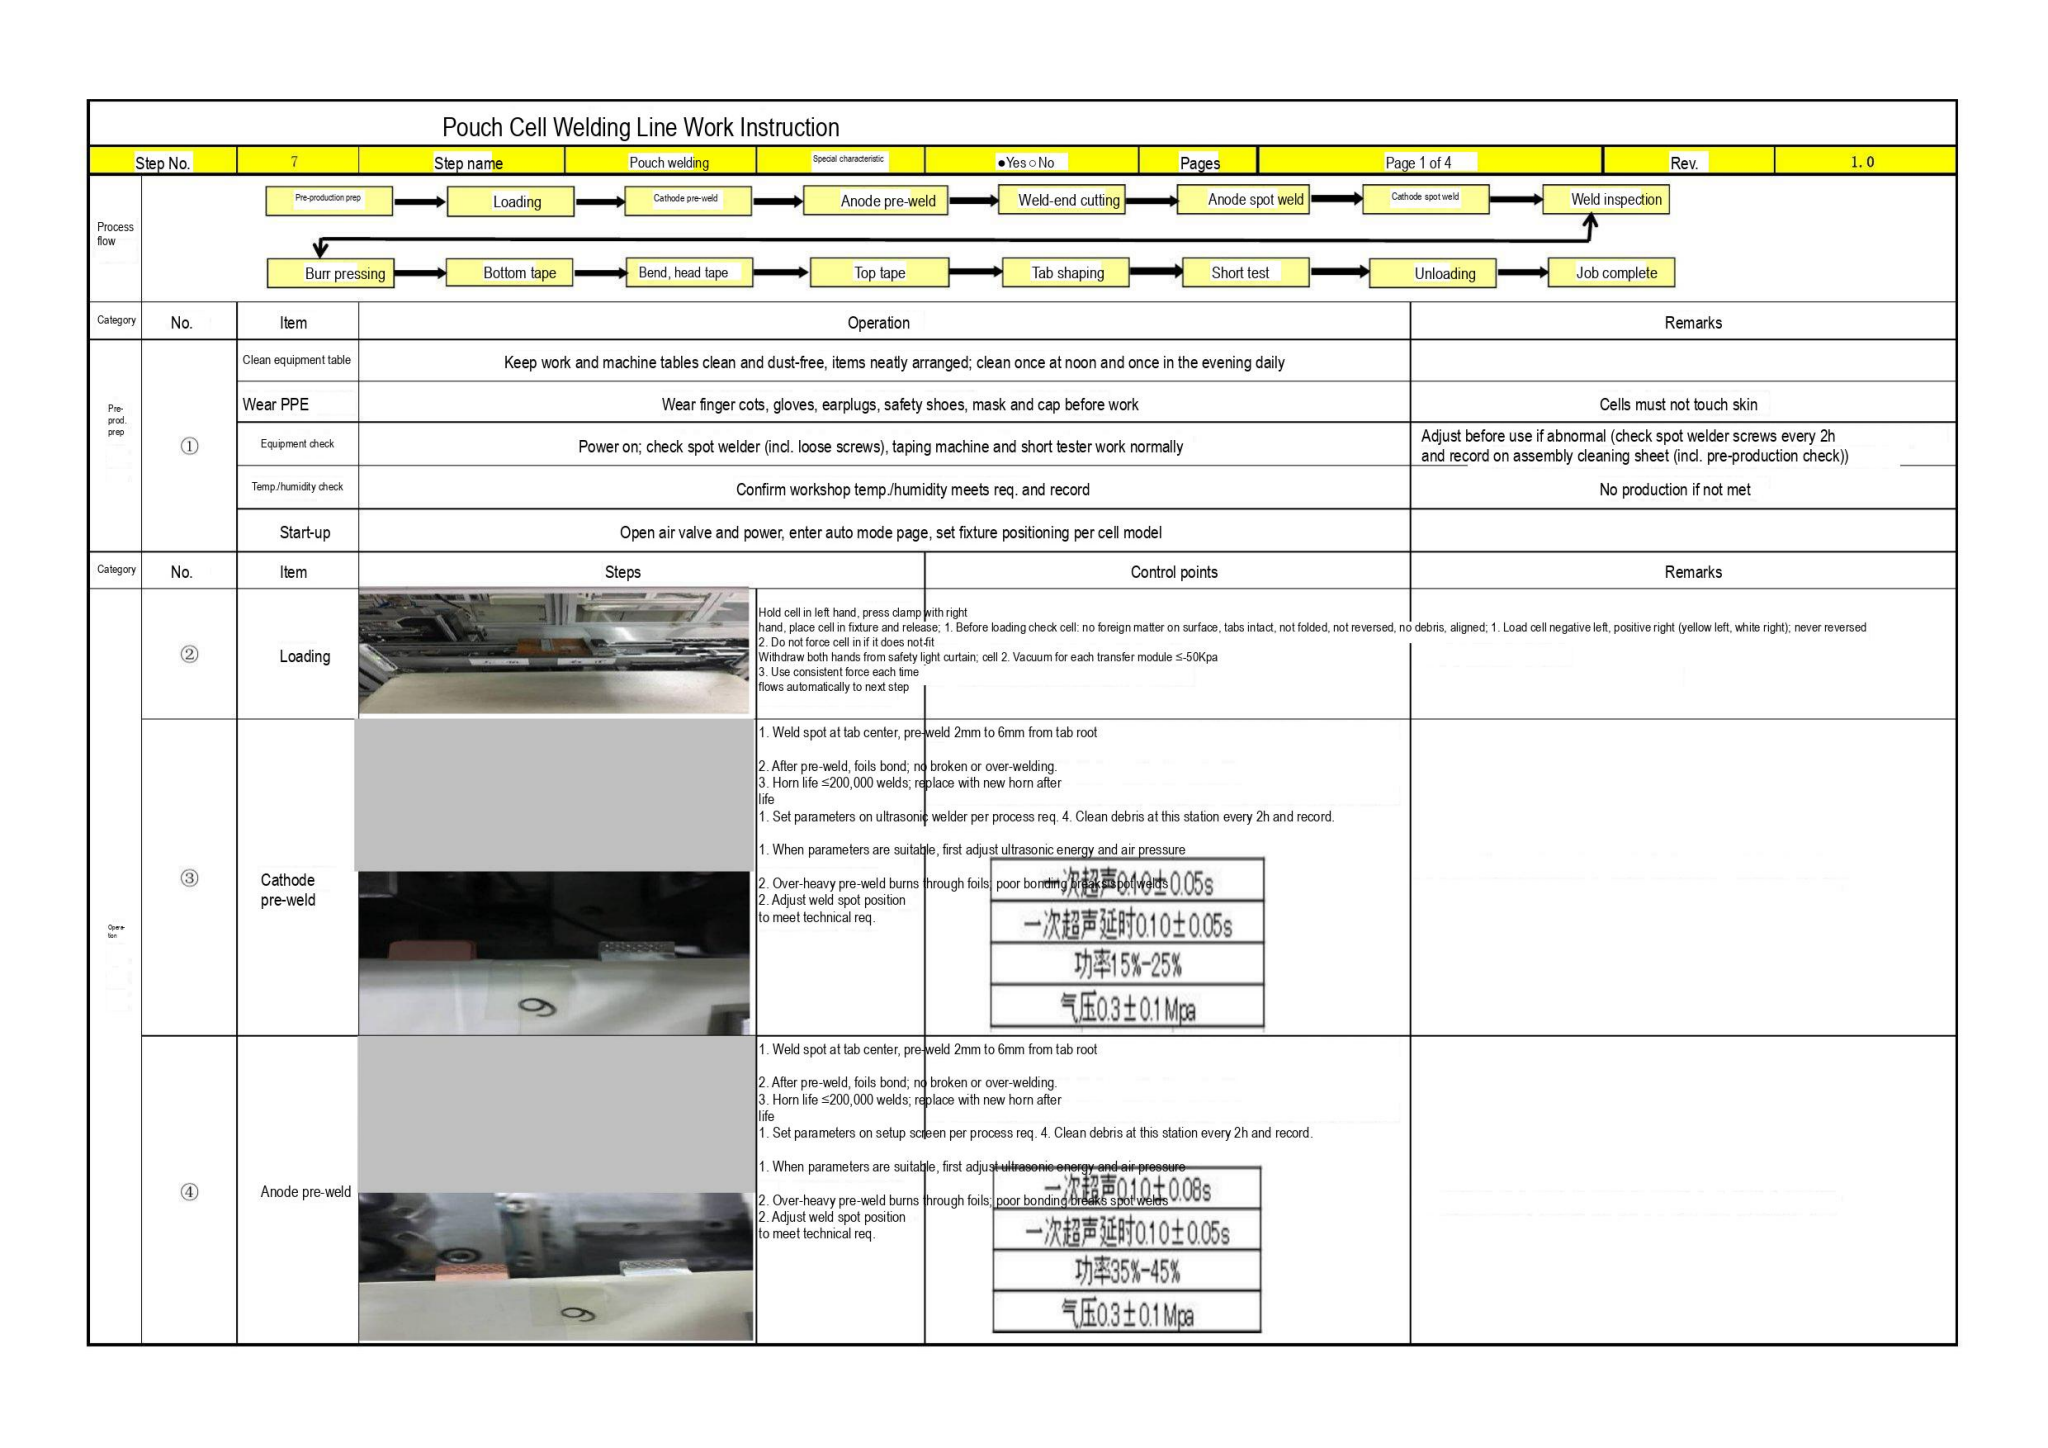# Pouch Cell Welding Line Work Instruction

| Step No. | 7 | Step name | Pouch welding | Special characteristic | ●Yes○No | Pages | Page 1 of 4 | Rev. | 1.0 |
|---|---|---|---|---|---|---|---|---|---|

Process flow

Pre-production prep → Loading → Cathode pre-weld → Anode pre-weld → Weld-end cutting → Anode spot weld → Cathode spot weld → Weld inspection

Burr pressing → Bottom tape → Bend, head tape → Top tape → Tab shaping → Short test → Unloading → Job complete

| Category | No. | Item | Operation | Remarks |
|---|---|---|---|---|
| Pre-prod. prep | ① | Clean equipment table | Keep work and machine tables clean and dust-free, items neatly arranged; clean once at noon and once in the evening daily | |
| | | Wear PPE | Wear finger cots, gloves, earplugs, safety shoes, mask and cap before work | Cells must not touch skin |
| | | Equipment check | Power on; check spot welder (incl. loose screws), taping machine and short tester work normally | Adjust before use if abnormal (check spot welder screws every 2h and record on assembly cleaning sheet (incl. pre-production check)) |
| | | Temp./humidity check | Confirm workshop temp./humidity meets req. and record | No production if not met |
| | | Start-up | Open air valve and power, enter auto mode page, set fixture positioning per cell model | |

| Category | No. | Item | Steps | Control points | Remarks |
|---|---|---|---|---|---|
| Opera-tion | ② | Loading | Hold cell in left hand, press clamp with right<br>hand, place cell in fixture and release; 1. Before loading check cell: no foreign matter on surface, tabs intact, not folded, not reversed, no debris, aligned; 1. Load cell negative left, positive right (yellow left, white right); never reversed<br>2. Do not force cell in if it does not fit<br>Withdraw both hands from safety light curtain; cell 2. Vacuum for each transfer module ≤-50Kpa<br>3. Use consistent force each time<br>flows automatically to next step | | |
| | ③ | Cathode pre-weld | 1. Weld spot at tab center, pre-weld 2mm to 6mm from tab root<br>2. After pre-weld, foils bond; no broken or over-welding.<br>3. Horn life ≤200,000 welds; replace with new horn after life<br>1. Set parameters on ultrasonic welder per process req. 4. Clean debris at this station every 2h and record.<br>1. When parameters are suitable, first adjust ultrasonic energy and air pressure<br>2. Over-heavy pre-weld burns through foils; poor bonding breaks spot welds<br>2. Adjust weld spot position to meet technical req. | 一次超声0.10±0.05s<br>一次超声延时0.10±0.05s<br>功率15%-25%<br>气压0.3±0.1Mpa | |
| | ④ | Anode pre-weld | 1. Weld spot at tab center, pre-weld 2mm to 6mm from tab root<br>2. After pre-weld, foils bond; no broken or over-welding.<br>3. Horn life ≤200,000 welds; replace with new horn after life<br>1. Set parameters on setup screen per process req. 4. Clean debris at this station every 2h and record.<br>1. When parameters are suitable, first adjust ultrasonic energy and air pressure<br>2. Over-heavy pre-weld burns through foils; poor bonding breaks spot welds<br>2. Adjust weld spot position to meet technical req. | 一次超声0.10±0.08s<br>一次超声延时0.10±0.05s<br>功率35%-45%<br>气压0.3±0.1Mpa | |
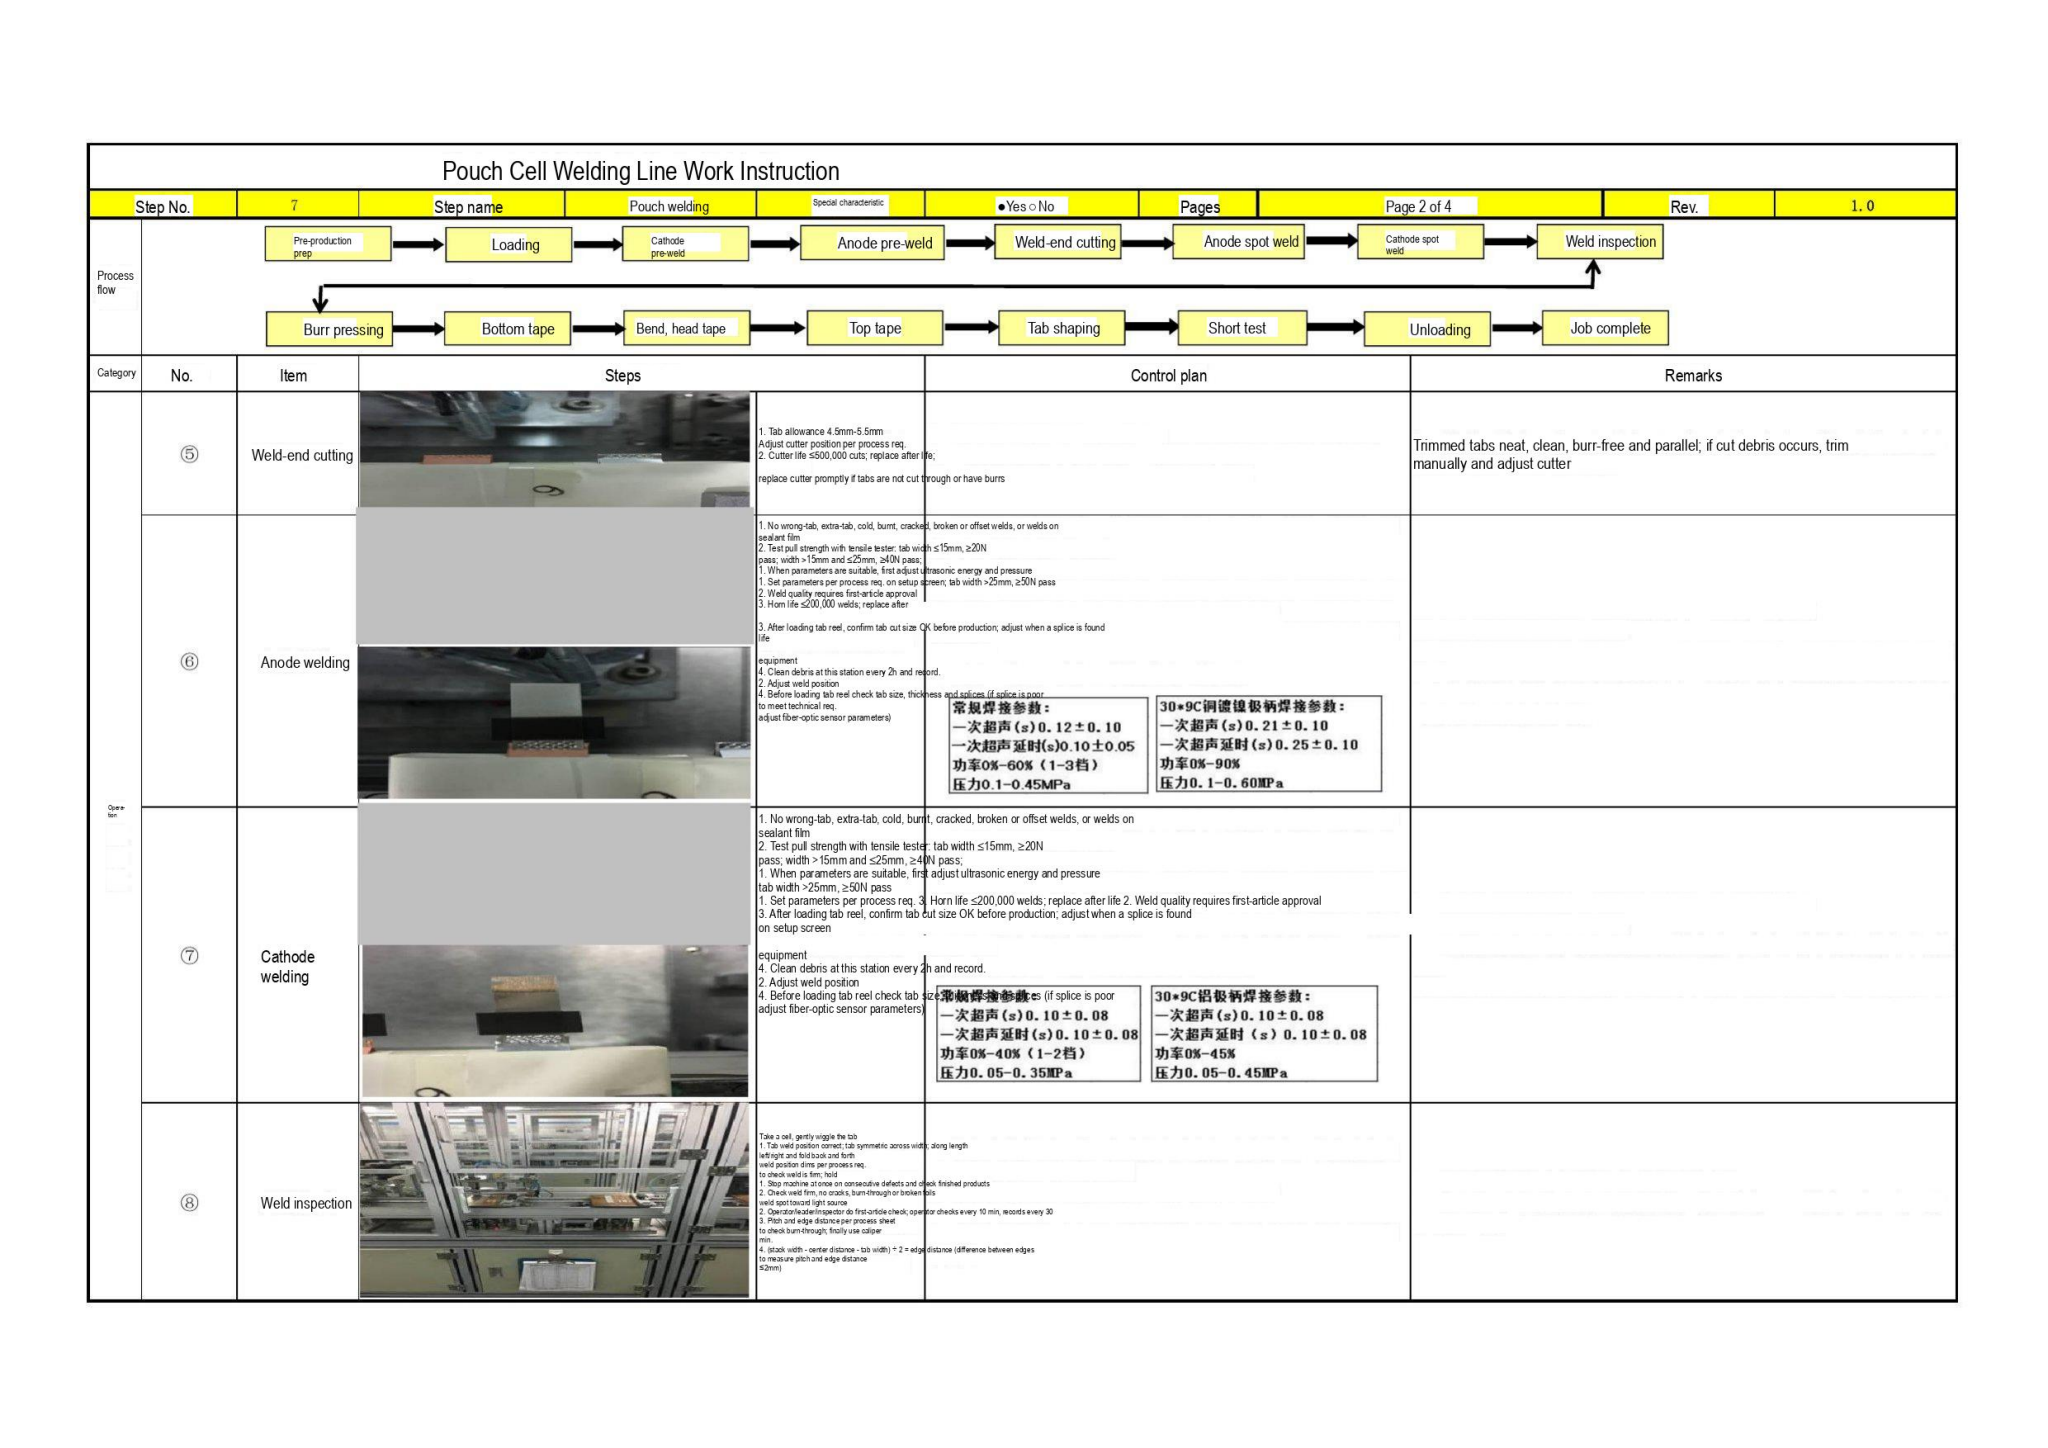Pouch Cell Welding Line Work Instruction

| Step No. | 7 | Step name | Pouch welding | Special characteristic | ●Yes ○No | Pages | Page 2 of 4 | Rev. | 1.0 |
|---|---|---|---|---|---|---|---|---|---|

Process flow

Pre-production prep → Loading → Cathode pre-weld → Anode pre-weld → Weld-end cutting → Anode spot weld → Cathode spot weld → Weld inspection → Burr pressing → Bottom tape → Bend, head tape → Top tape → Tab shaping → Short test → Unloading → Job complete

| Category | No. | Item | Steps | Control plan | Remarks |
|---|---|---|---|---|---|
| Operation | ⑤ | Weld-end cutting | | 1. Tab allowance 4.5mm-5.5mm<br>Adjust cutter position per process req.<br>2. Cutter life ≤500,000 cuts; replace after life;<br><br>replace cutter promptly if tabs are not cut through or have burrs | Trimmed tabs neat, clean, burr-free and parallel; if cut debris occurs, trim manually and adjust cutter |
| | ⑥ | Anode welding | | 1. No wrong-tab, extra-tab, cold, burnt, cracked, broken or offset welds, or welds on sealant film<br>2. Test pull strength with tensile tester: tab width ≤15mm, ≥20N pass; width >15mm and ≤25mm, ≥40N pass;<br>1. When parameters are suitable, first adjust ultrasonic energy and pressure<br>1. Set parameters per process req. on setup screen; tab width >25mm, ≥50N pass<br>2. Weld quality requires first-article approval<br>3. Horn life ≤200,000 welds; replace after<br><br>3. After loading tab reel, confirm tab cut size OK before production; adjust when a splice is found<br>life<br><br>equipment<br>4. Clean debris at this station every 2h and record.<br>2. Adjust weld position<br>4. Before loading tab reel check tab size, thickness and splices (if splice is poor<br>to meet technical req.<br>adjust fiber-optic sensor parameters)<br><br>常规焊接参数：<br>一次超声(s)0.12±0.10<br>一次超声延时(s)0.10±0.05<br>功率0%-60%（1-3档）<br>压力0.1-0.45MPa<br><br>30*9C铜镀镍极柄焊接参数：<br>一次超声(s)0.21±0.10<br>一次超声延时(s)0.25±0.10<br>功率0%-90%<br>压力0.1-0.60MPa | |
| | ⑦ | Cathode welding | | 1. No wrong-tab, extra-tab, cold, burnt, cracked, broken or offset welds, or welds on sealant film<br>2. Test pull strength with tensile tester: tab width ≤15mm, ≥20N pass; width >15mm and ≤25mm, ≥40N pass;<br>1. When parameters are suitable, first adjust ultrasonic energy and pressure<br>tab width >25mm, ≥50N pass<br>1. Set parameters per process req. 3. Horn life ≤200,000 welds; replace after life 2. Weld quality requires first-article approval<br>3. After loading tab reel, confirm tab cut size OK before production; adjust when a splice is found<br>on setup screen<br><br>equipment<br>4. Clean debris at this station every 2h and record.<br>2. Adjust weld position<br>4. Before loading tab reel check tab size (if splice is poor<br>adjust fiber-optic sensor parameters)<br><br>常规焊接参数：<br>一次超声(s)0.10±0.08<br>一次超声延时(s)0.10±0.08<br>功率0%-40%（1-2档）<br>压力0.05-0.35MPa<br><br>30*9C铝极柄焊接参数：<br>一次超声(s)0.10±0.08<br>一次超声延时（s）0.10±0.08<br>功率0%-45%<br>压力0.05-0.45MPa | |
| | ⑧ | Weld inspection | | Take a cell, gently wiggle the tab<br>1. Tab weld position correct; tab symmetric across width; along length<br>left/right and fold back and forth<br>weld position dims per process req.<br>to check weld is firm; hold<br>1. Stop machine at once on consecutive defects and check finished products<br>2. Check weld firm, no cracks, burn-through or broken foils<br>weld spot toward light source<br>2. Operator/leader/inspector do first-article check; operator checks every 10 min, records every 30<br>3. Pitch and edge distance per process sheet<br>to check burn-through; finally use caliper<br>min.<br>4. (stack width - center distance - tab width) ÷ 2 = edge distance (difference between edges<br>to measure pitch and edge distance<br>≤2mm) | |
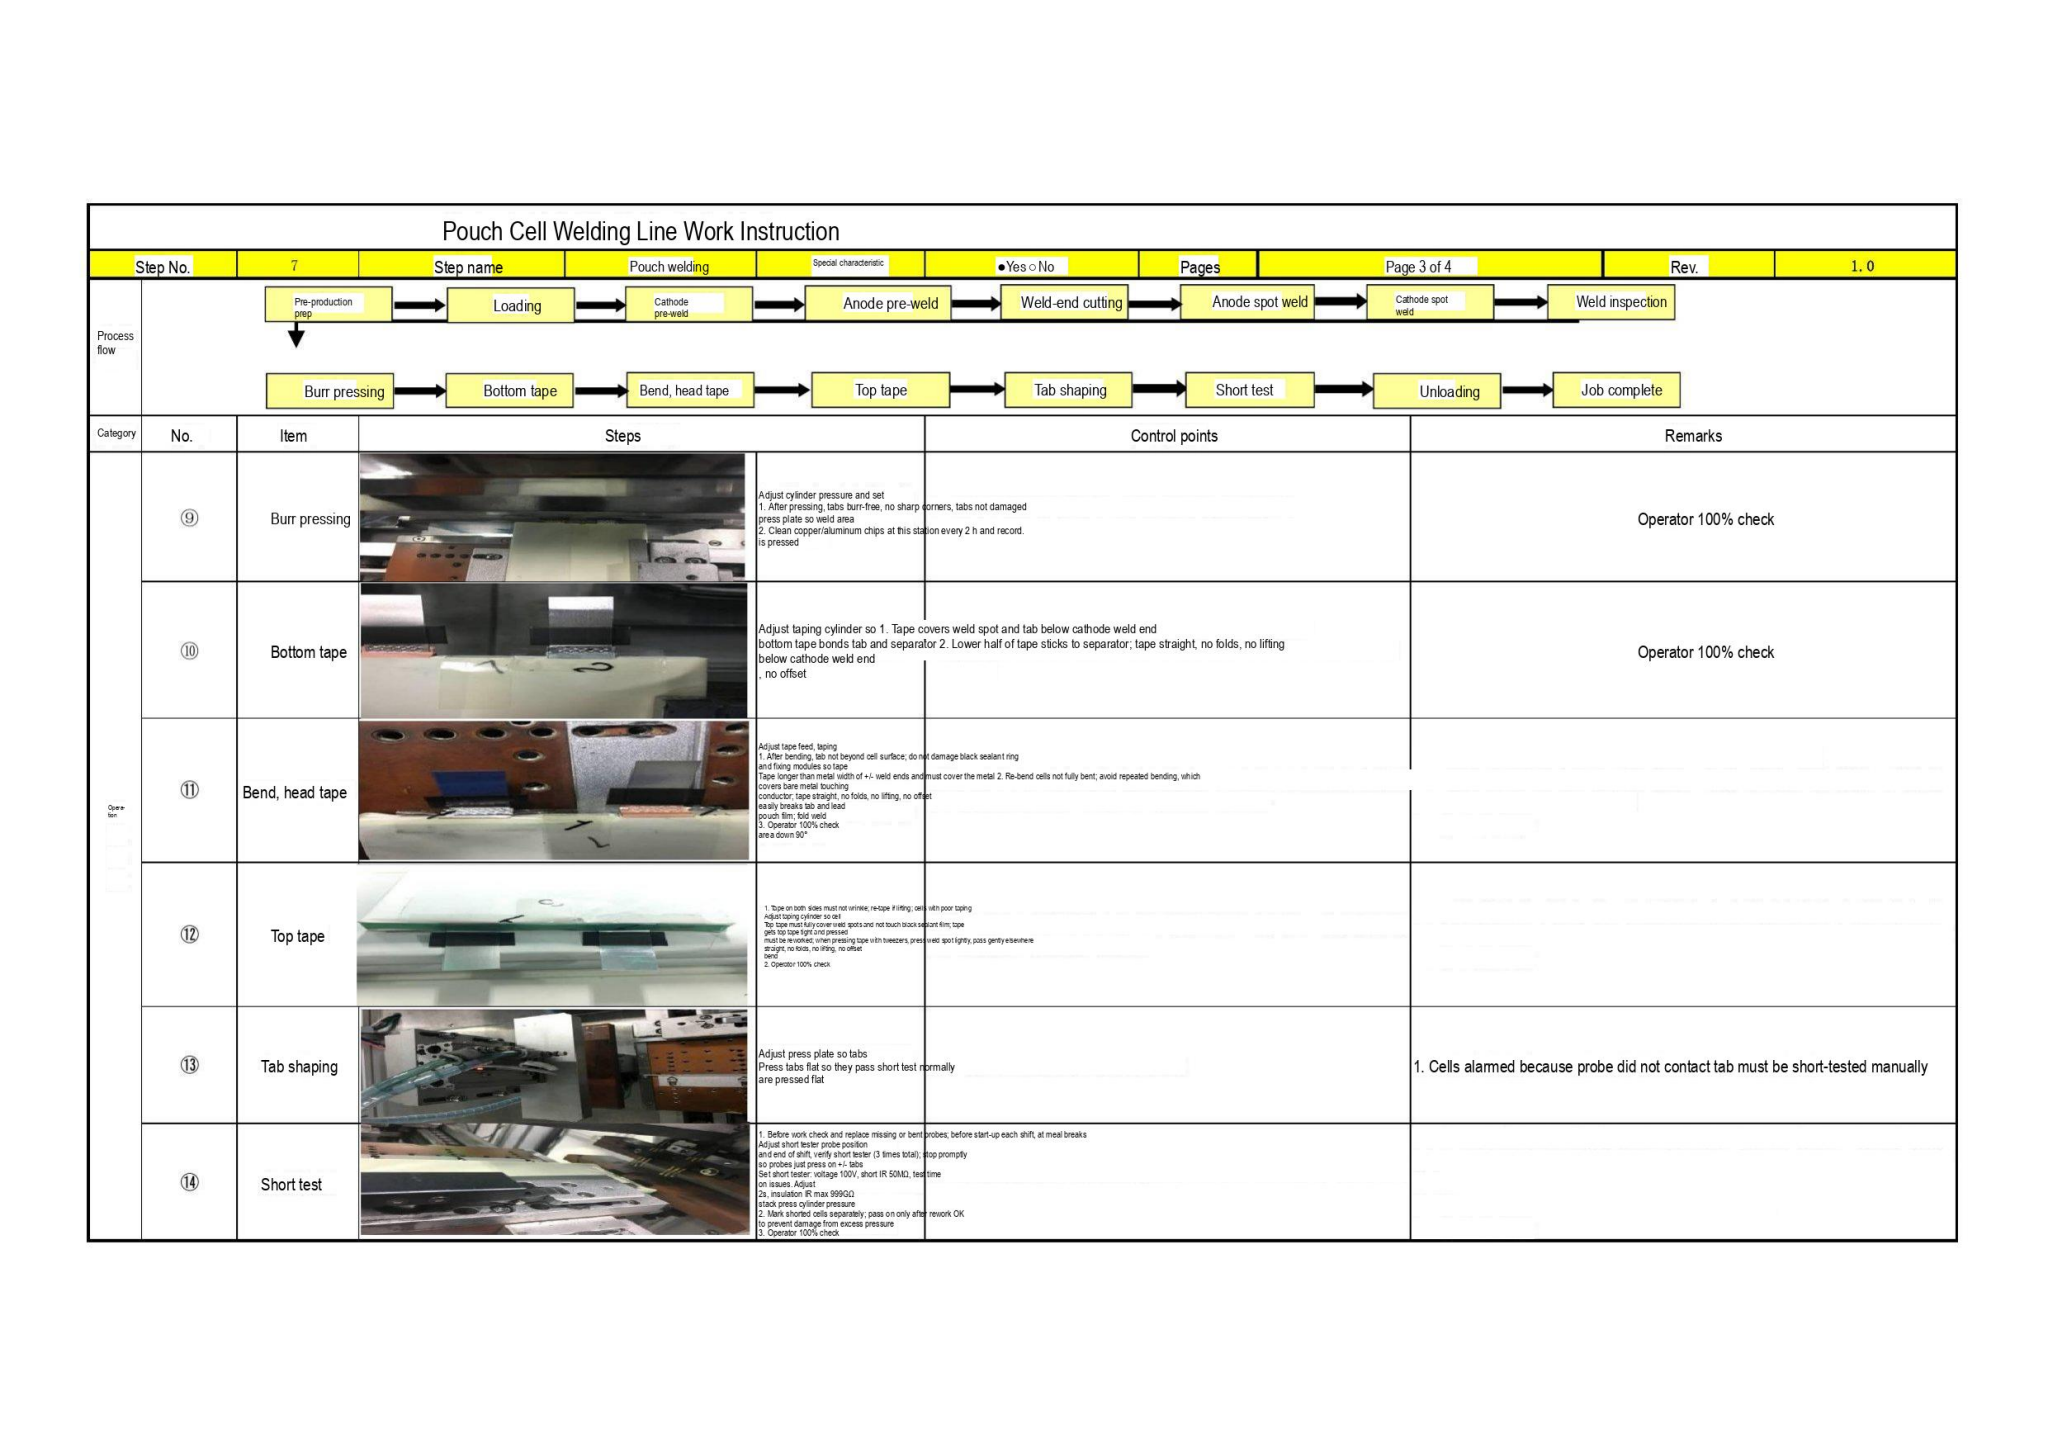Pouch Cell Welding Line Work Instruction

| Step No. | 7 | Step name | Pouch welding | Special characteristic | ●Yes ○No | Pages | Page 3 of 4 | Rev. | 1. 0 |
|---|---|---|---|---|---|---|---|---|---|

Process flow

Pre-production prep → Loading → Cathode pre-weld → Anode pre-weld → Weld-end cutting → Anode spot weld → Cathode spot weld → Weld inspection

Burr pressing → Bottom tape → Bend, head tape → Top tape → Tab shaping → Short test → Unloading → Job complete

| Category | No. | Item | Steps | Control points | Remarks |
|---|---|---|---|---|---|
| Operation | ⑨ | Burr pressing | Adjust cylinder pressure and set press plate so weld area is pressed | 1. After pressing, tabs burr-free, no sharp corners, tabs not damaged<br>2. Clean copper/aluminum chips at this station every 2 h and record. | Operator 100% check |
| | ⑩ | Bottom tape | Adjust taping cylinder so bottom tape bonds tab and separator below cathode weld end, no offset | 1. Tape covers weld spot and tab below cathode weld end<br>2. Lower half of tape sticks to separator; tape straight, no folds, no lifting | Operator 100% check |
| | ⑪ | Bend, head tape | Adjust tape feed, taping and fixing modules so tape covers bare metal touching conductor; tape straight, no folds, no lifting, no offset<br>Tape longer than metal width of +/- weld ends and pouch film; fold weld area down 90° | 1. After bending, tab not beyond cell surface; do not damage black sealant ring<br>must cover the metal 2. Re-bend cells not fully bent; avoid repeated bending, which easily breaks tab and lead<br>3. Operator 100% check | |
| | ⑫ | Top tape | Adjust taping cylinder so cell gets top tape tight and pressed straight, no folds, no lifting, no offset | 1. Tape on both sides must not wrinkle; re-tape if lifting; cells with poor taping must be reworked; when pressing tape with tweezers, press weld spot lightly, pass gently elsewhere<br>Top tape must fully cover weld spots and not touch black sealant film; tape bend<br>2. Operator 100% check | |
| | ⑬ | Tab shaping | Adjust press plate so tabs are pressed flat | Press tabs flat so they pass short test normally | 1. Cells alarmed because probe did not contact tab must be short-tested manually |
| | ⑭ | Short test | Adjust short tester probe position so probes just press on +/- tabs<br>Set short tester: voltage 100V, short IR 50MΩ, test time 2s, insulation IR max 999GΩ<br>Adjust stack press cylinder pressure to prevent damage from excess pressure | 1. Before work check and replace missing or bent probes; before start-up each shift, at meal breaks and end of shift, verify short tester (3 times total); stop promptly on issues.<br>2. Mark shorted cells separately; pass on only after rework OK<br>3. Operator 100% check | |
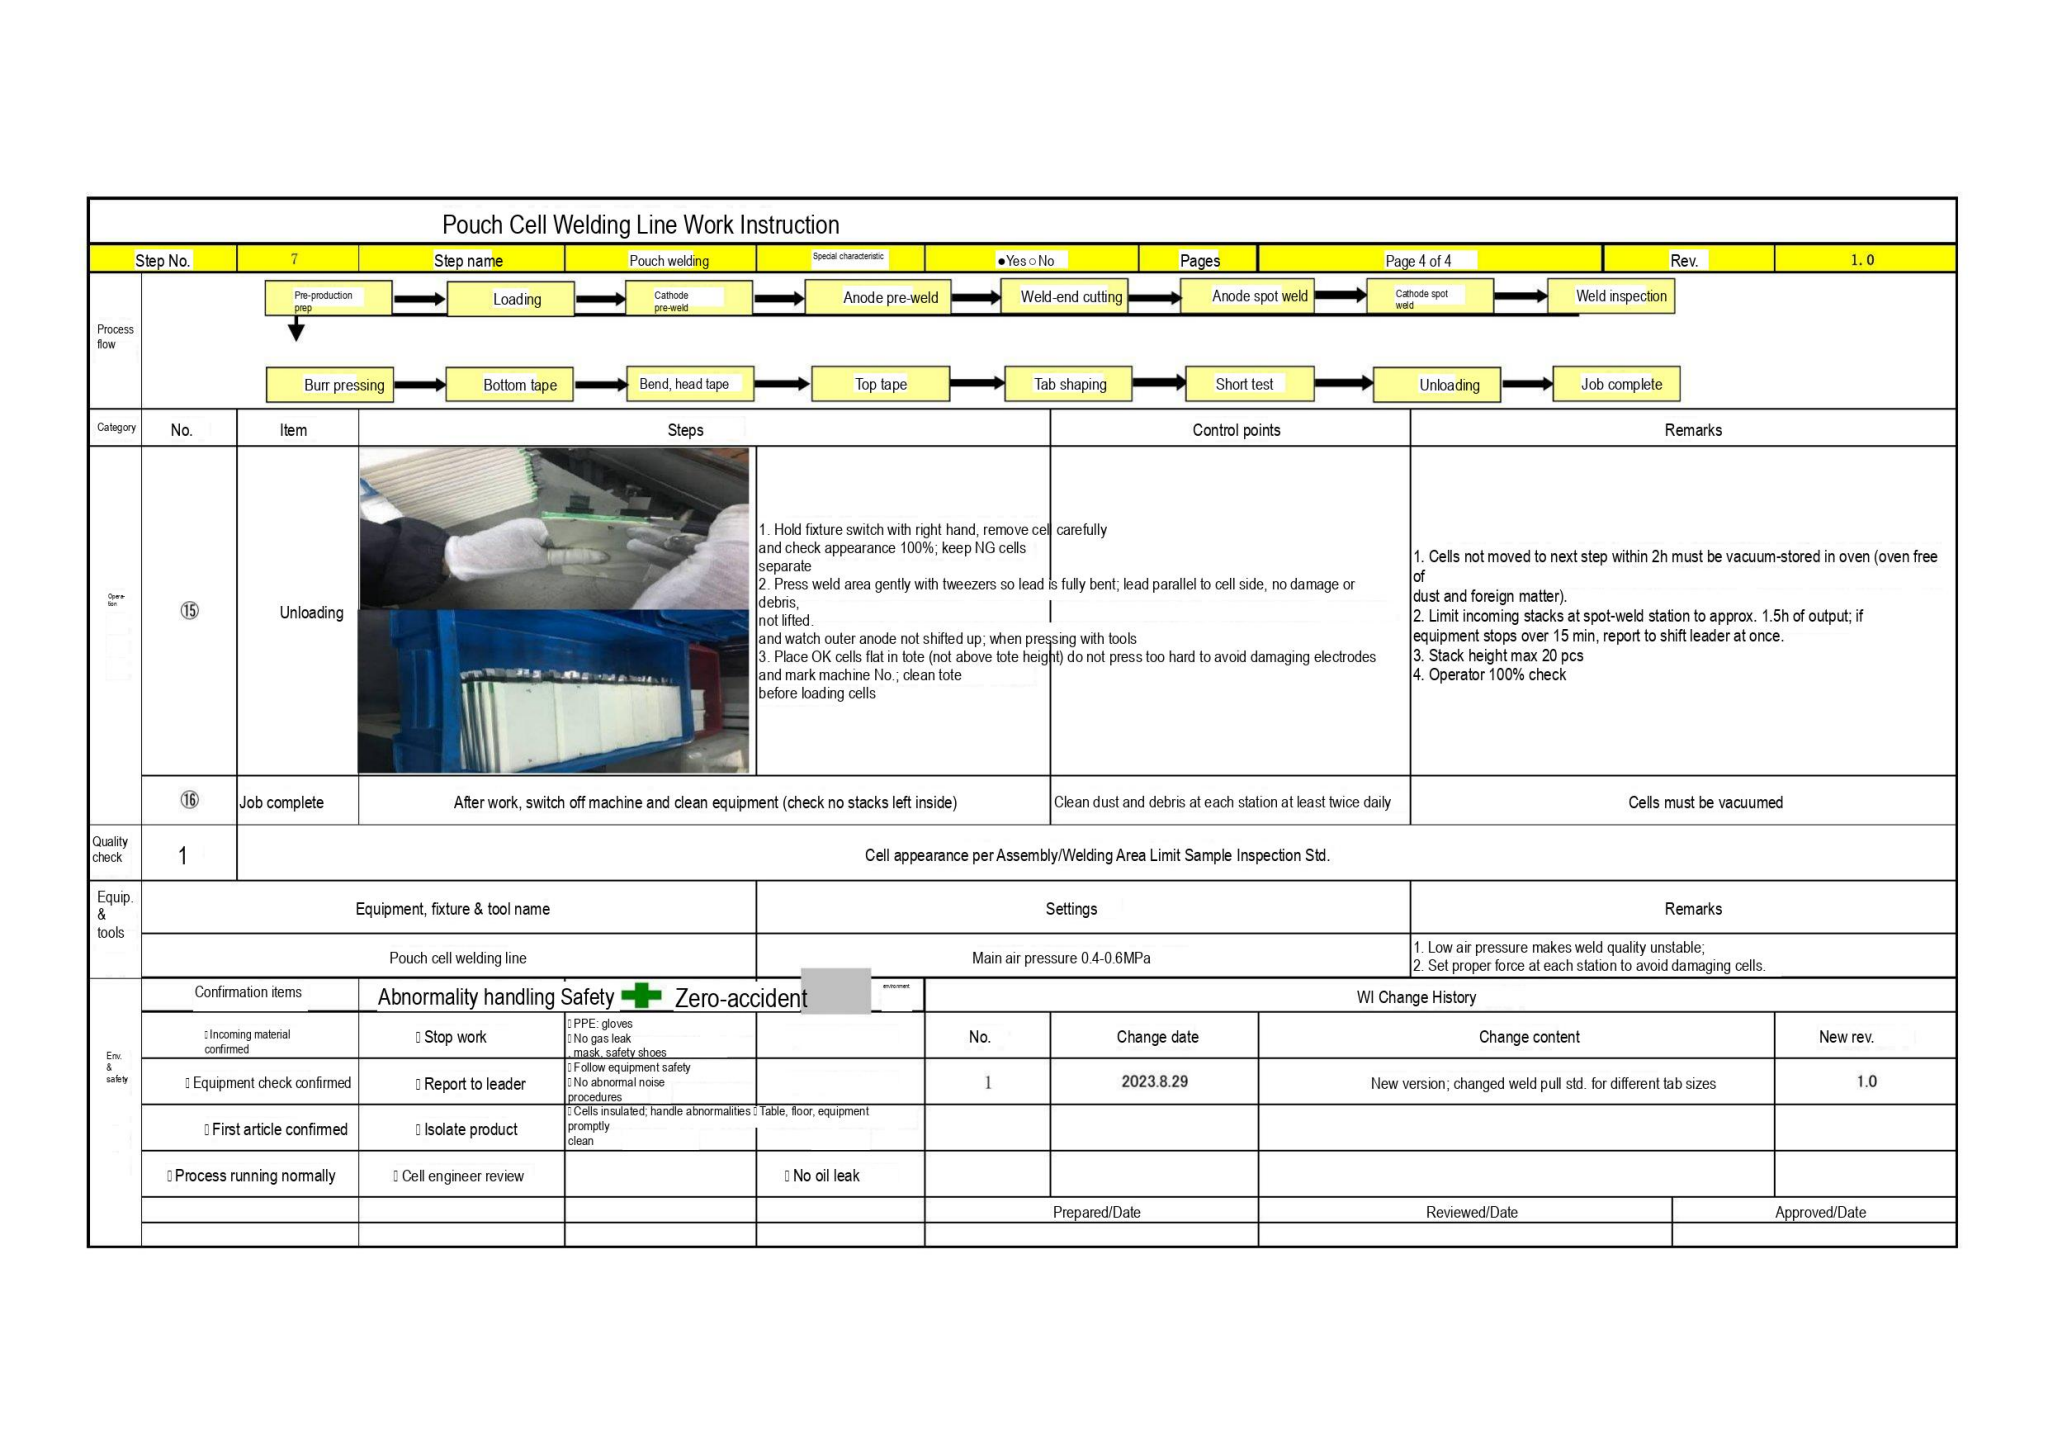Pouch Cell Welding Line Work Instruction

| Step No. | 7 | Step name | Pouch welding | Special characteristic | ●Yes ○No | Pages | Page 4 of 4 | Rev. | 1.0 |
|---|---|---|---|---|---|---|---|---|---|

Process flow

Pre-production prep → Loading → Cathode pre-weld → Anode pre-weld → Weld-end cutting → Anode spot weld → Cathode spot weld → Weld inspection

Burr pressing → Bottom tape → Bend, head tape → Top tape → Tab shaping → Short test → Unloading → Job complete

| Category | No. | Item | Steps | Control points | Remarks |
|---|---|---|---|---|---|
| Operation | ⑮ | Unloading | 1. Hold fixture switch with right hand, remove cell carefully and check appearance 100%; keep NG cells separate<br>2. Press weld area gently with tweezers so lead is fully bent; lead parallel to cell side, no damage or debris, not lifted.<br>and watch outer anode not shifted up; when pressing with tools<br>3. Place OK cells flat in tote (not above tote height) do not press too hard to avoid damaging electrodes and mark machine No.; clean tote before loading cells | | 1. Cells not moved to next step within 2h must be vacuum-stored in oven (oven free of dust and foreign matter).<br>2. Limit incoming stacks at spot-weld station to approx. 1.5h of output; if equipment stops over 15 min, report to shift leader at once.<br>3. Stack height max 20 pcs<br>4. Operator 100% check |
| | ⑯ | Job complete | After work, switch off machine and clean equipment (check no stacks left inside) | Clean dust and debris at each station at least twice daily | Cells must be vacuumed |
| Quality check | 1 | Cell appearance per Assembly/Welding Area Limit Sample Inspection Std. | | | |

| Equip. & tools | Equipment, fixture & tool name | Settings | Remarks |
|---|---|---|---|
| | Pouch cell welding line | Main air pressure 0.4-0.6MPa | 1. Low air pressure makes weld quality unstable;<br>2. Set proper force at each station to avoid damaging cells. |

| Env. & safety | Confirmation items | Abnormality handling | Safety | Zero-accident | environment | WI Change History | | | |
|---|---|---|---|---|---|---|---|---|---|
| | | | | | | No. | Change date | Change content | New rev. |
| | Incoming material confirmed | Stop work | PPE: gloves<br>No gas leak<br>mask, safety shoes | | | | | | |
| | Equipment check confirmed | Report to leader | Follow equipment safety<br>No abnormal noise<br>procedures | | | 1 | 2023.8.29 | New version; changed weld pull std. for different tab sizes | 1.0 |
| | First article confirmed | Isolate product | Cells insulated; handle abnormalities promptly | Table, floor, equipment clean | | | | | |
| | Process running normally | Cell engineer review | | No oil leak | | | | | |
| | | | | | | Prepared/Date | | Reviewed/Date | Approved/Date |